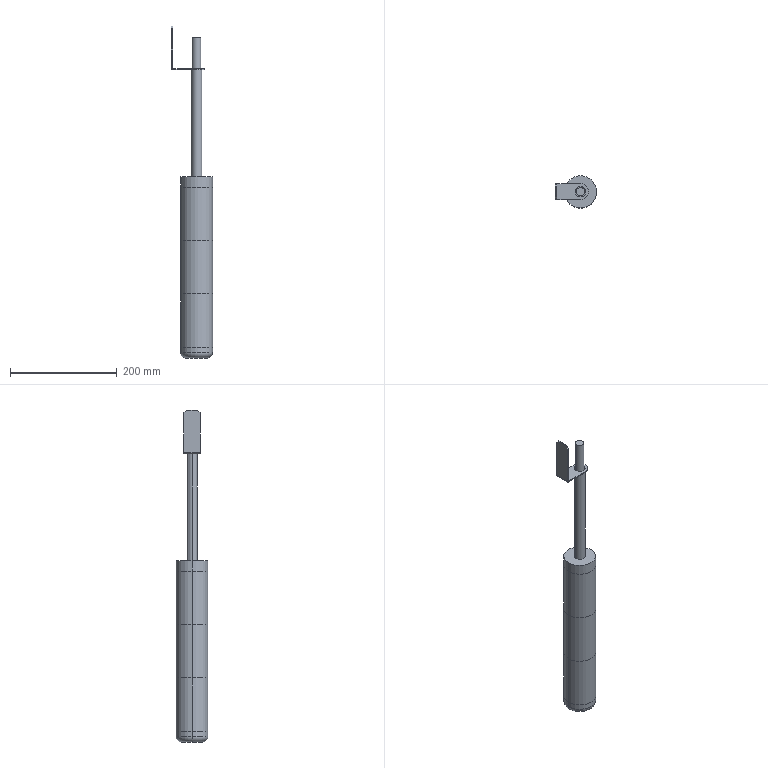Part | SolidWorks | features BaseBody 6 | 6 solids | 47 faces | box 77 x 60 x 622 mm | volume 1040083 mm3 | plane 25 | cylinder 20 | torus 2 | commonest cylinder face diameters 60 x10 20 x4 16 x2 30 x2 1.473 x1 5.473 x1
STEP:
#1=CARTESIAN_POINT('',(-20.,0.,0.));
#2=VERTEX_POINT('',#1);
#3=CARTESIAN_POINT('',(20.,0.,0.));
#4=VERTEX_POINT('',#3);
#5=CARTESIAN_POINT('',(0.,0.,0.));
#6=DIRECTION('',(0.,0.,-1.));
#7=DIRECTION('',(1.,0.,0.));
#8=AXIS2_PLACEMENT_3D('',#5,#6,#7);
#9=CIRCLE('',#8,20.);
#10=EDGE_CURVE('',#2,#4,#9,.T.);
#11=ORIENTED_EDGE('',*,*,#10,.F.);
#12=CARTESIAN_POINT('',(-30.,0.,10.));
#13=VERTEX_POINT('',#12);
#14=CARTESIAN_POINT('',(-20.,0.,10.));
#15=DIRECTION('',(0.,1.,0.));
#16=DIRECTION('',(-1.,0.,0.));
#17=AXIS2_PLACEMENT_3D('',#14,#15,#16);
#18=CIRCLE('',#17,10.);
#19=EDGE_CURVE('',#2,#13,#18,.T.);
#20=ORIENTED_EDGE('',*,*,#19,.T.);
#21=CARTESIAN_POINT('',(30.,0.,10.));
#22=VERTEX_POINT('',#21);
#23=CARTESIAN_POINT('',(0.,0.,10.));
#24=DIRECTION('',(0.,0.,1.));
#25=DIRECTION('',(1.,0.,0.));
#26=AXIS2_PLACEMENT_3D('',#23,#24,#25);
#27=CIRCLE('',#26,30.);
#28=EDGE_CURVE('',#22,#13,#27,.T.);
#29=ORIENTED_EDGE('',*,*,#28,.F.);
#30=CARTESIAN_POINT('',(20.,0.,10.));
#31=DIRECTION('',(0.,-1.,0.));
#32=DIRECTION('',(0.,0.,-1.));
#33=AXIS2_PLACEMENT_3D('',#30,#31,#32);
#34=CIRCLE('',#33,10.);
#35=EDGE_CURVE('',#4,#22,#34,.T.);
#36=ORIENTED_EDGE('',*,*,#35,.F.);
#37=EDGE_LOOP('',(#11,#20,#29,#36));
#38=FACE_OUTER_BOUND('',#37,.T.);
#39=CARTESIAN_POINT('',(0.,0.,10.));
#40=DIRECTION('',(0.,0.,1.));
#41=DIRECTION('',(1.,0.,0.));
#42=AXIS2_PLACEMENT_3D('',#39,#40,#41);
#43=TOROIDAL_SURFACE('',#42,20.,10.);
#44=ADVANCED_FACE('',(#38),#43,.T.);
#45=CARTESIAN_POINT('',(30.,0.,20.));
#46=VERTEX_POINT('',#45);
#47=CARTESIAN_POINT('',(-30.,0.,20.));
#48=VERTEX_POINT('',#47);
#49=CARTESIAN_POINT('',(0.,0.,20.));
#50=DIRECTION('',(0.,0.,1.));
#51=DIRECTION('',(1.,0.,0.));
#52=AXIS2_PLACEMENT_3D('',#49,#50,#51);
#53=CIRCLE('',#52,30.);
#54=EDGE_CURVE('',#46,#48,#53,.T.);
#55=ORIENTED_EDGE('',*,*,#54,.F.);
#56=CARTESIAN_POINT('',(30.,0.,20.));
#57=DIRECTION('',(0.,0.,-1.));
#58=VECTOR('',#57,1000.);
#59=LINE('',#56,#58);
#60=EDGE_CURVE('',#46,#22,#59,.T.);
#61=ORIENTED_EDGE('',*,*,#60,.T.);
#62=ORIENTED_EDGE('',*,*,#28,.T.);
#63=CARTESIAN_POINT('',(-30.,0.,20.));
#64=DIRECTION('',(0.,0.,-1.));
#65=VECTOR('',#64,1000.);
#66=LINE('',#63,#65);
#67=EDGE_CURVE('',#48,#13,#66,.T.);
#68=ORIENTED_EDGE('',*,*,#67,.F.);
#69=EDGE_LOOP('',(#55,#61,#62,#68));
#70=FACE_OUTER_BOUND('',#69,.T.);
#71=CARTESIAN_POINT('',(0.,0.,20.));
#72=DIRECTION('',(0.,0.,-1.));
#73=DIRECTION('',(-1.,0.,0.));
#74=AXIS2_PLACEMENT_3D('',#71,#72,#73);
#75=CYLINDRICAL_SURFACE('',#74,30.);
#76=ADVANCED_FACE('',(#70),#75,.T.);
#77=ORIENTED_EDGE('',*,*,#60,.F.);
#78=CARTESIAN_POINT('',(0.,0.,20.));
#79=DIRECTION('',(0.,0.,1.));
#80=DIRECTION('',(1.,0.,0.));
#81=AXIS2_PLACEMENT_3D('',#78,#79,#80);
#82=CIRCLE('',#81,30.);
#83=EDGE_CURVE('',#48,#46,#82,.T.);
#84=ORIENTED_EDGE('',*,*,#83,.F.);
#85=ORIENTED_EDGE('',*,*,#67,.T.);
#86=CARTESIAN_POINT('',(0.,0.,10.));
#87=DIRECTION('',(0.,0.,1.));
#88=DIRECTION('',(1.,0.,0.));
#89=AXIS2_PLACEMENT_3D('',#86,#87,#88);
#90=CIRCLE('',#89,30.);
#91=EDGE_CURVE('',#13,#22,#90,.T.);
#92=ORIENTED_EDGE('',*,*,#91,.T.);
#93=EDGE_LOOP('',(#77,#84,#85,#92));
#94=FACE_OUTER_BOUND('',#93,.T.);
#95=CARTESIAN_POINT('',(0.,0.,20.));
#96=DIRECTION('',(0.,0.,-1.));
#97=DIRECTION('',(-1.,0.,0.));
#98=AXIS2_PLACEMENT_3D('',#95,#96,#97);
#99=CYLINDRICAL_SURFACE('',#98,30.);
#100=ADVANCED_FACE('',(#94),#99,.T.);
#101=ORIENTED_EDGE('',*,*,#83,.T.);
#102=ORIENTED_EDGE('',*,*,#54,.T.);
#103=EDGE_LOOP('',(#101,#102));
#104=FACE_OUTER_BOUND('',#103,.T.);
#105=CARTESIAN_POINT('',(0.,0.,20.));
#106=DIRECTION('',(0.,0.,1.));
#107=DIRECTION('',(1.,0.,0.));
#108=AXIS2_PLACEMENT_3D('',#105,#106,#107);
#109=PLANE('',#108);
#110=ADVANCED_FACE('',(#104),#109,.T.);
#111=CARTESIAN_POINT('',(0.,0.,0.));
#112=DIRECTION('',(0.,0.,-1.));
#113=DIRECTION('',(1.,0.,0.));
#114=AXIS2_PLACEMENT_3D('',#111,#112,#113);
#115=CIRCLE('',#114,20.);
#116=EDGE_CURVE('',#4,#2,#115,.T.);
#117=ORIENTED_EDGE('',*,*,#116,.T.);
#118=ORIENTED_EDGE('',*,*,#10,.T.);
#119=EDGE_LOOP('',(#117,#118));
#120=FACE_OUTER_BOUND('',#119,.T.);
#121=CARTESIAN_POINT('',(0.,0.,0.));
#122=DIRECTION('',(0.,0.,1.));
#123=DIRECTION('',(1.,0.,0.));
#124=AXIS2_PLACEMENT_3D('',#121,#122,#123);
#125=PLANE('',#124);
#126=ADVANCED_FACE('',(#120),#125,.F.);
#127=ORIENTED_EDGE('',*,*,#19,.F.);
#128=ORIENTED_EDGE('',*,*,#116,.F.);
#129=ORIENTED_EDGE('',*,*,#35,.T.);
#130=ORIENTED_EDGE('',*,*,#91,.F.);
#131=EDGE_LOOP('',(#127,#128,#129,#130));
#132=FACE_OUTER_BOUND('',#131,.T.);
#133=CARTESIAN_POINT('',(0.,0.,10.));
#134=DIRECTION('',(0.,0.,1.));
#135=DIRECTION('',(1.,0.,0.));
#136=AXIS2_PLACEMENT_3D('',#133,#134,#135);
#137=TOROIDAL_SURFACE('',#136,20.,10.);
#138=ADVANCED_FACE('',(#132),#137,.T.);
#139=CLOSED_SHELL('',(#44,#76,#100,#110,#126,#138));
#140=MANIFOLD_SOLID_BREP('',#139);
#141=CARTESIAN_POINT('',(30.,0.,120.));
#142=VERTEX_POINT('',#141);
#143=CARTESIAN_POINT('',(-30.,0.,120.));
#144=VERTEX_POINT('',#143);
#145=CARTESIAN_POINT('',(0.,0.,120.));
#146=DIRECTION('',(0.,0.,1.));
#147=DIRECTION('',(1.,0.,0.));
#148=AXIS2_PLACEMENT_3D('',#145,#146,#147);
#149=CIRCLE('',#148,30.);
#150=EDGE_CURVE('',#142,#144,#149,.T.);
#151=ORIENTED_EDGE('',*,*,#150,.F.);
#152=CARTESIAN_POINT('',(30.,0.,20.));
#153=VERTEX_POINT('',#152);
#154=CARTESIAN_POINT('',(30.,0.,120.));
#155=DIRECTION('',(0.,0.,-1.));
#156=VECTOR('',#155,1000.);
#157=LINE('',#154,#156);
#158=EDGE_CURVE('',#142,#153,#157,.T.);
#159=ORIENTED_EDGE('',*,*,#158,.T.);
#160=CARTESIAN_POINT('',(-30.,0.,20.));
#161=VERTEX_POINT('',#160);
#162=CARTESIAN_POINT('',(0.,0.,20.));
#163=DIRECTION('',(0.,0.,1.));
#164=DIRECTION('',(1.,0.,0.));
#165=AXIS2_PLACEMENT_3D('',#162,#163,#164);
#166=CIRCLE('',#165,30.);
#167=EDGE_CURVE('',#153,#161,#166,.T.);
#168=ORIENTED_EDGE('',*,*,#167,.T.);
#169=CARTESIAN_POINT('',(-30.,0.,120.));
#170=DIRECTION('',(0.,0.,-1.));
#171=VECTOR('',#170,1000.);
#172=LINE('',#169,#171);
#173=EDGE_CURVE('',#144,#161,#172,.T.);
#174=ORIENTED_EDGE('',*,*,#173,.F.);
#175=EDGE_LOOP('',(#151,#159,#168,#174));
#176=FACE_OUTER_BOUND('',#175,.T.);
#177=CARTESIAN_POINT('',(0.,0.,120.));
#178=DIRECTION('',(0.,0.,-1.));
#179=DIRECTION('',(-1.,0.,0.));
#180=AXIS2_PLACEMENT_3D('',#177,#178,#179);
#181=CYLINDRICAL_SURFACE('',#180,30.);
#182=ADVANCED_FACE('',(#176),#181,.T.);
#183=ORIENTED_EDGE('',*,*,#158,.F.);
#184=CARTESIAN_POINT('',(0.,0.,120.));
#185=DIRECTION('',(0.,0.,1.));
#186=DIRECTION('',(1.,0.,0.));
#187=AXIS2_PLACEMENT_3D('',#184,#185,#186);
#188=CIRCLE('',#187,30.);
#189=EDGE_CURVE('',#144,#142,#188,.T.);
#190=ORIENTED_EDGE('',*,*,#189,.F.);
#191=ORIENTED_EDGE('',*,*,#173,.T.);
#192=CARTESIAN_POINT('',(0.,0.,20.));
#193=DIRECTION('',(0.,0.,1.));
#194=DIRECTION('',(1.,0.,0.));
#195=AXIS2_PLACEMENT_3D('',#192,#193,#194);
#196=CIRCLE('',#195,30.);
#197=EDGE_CURVE('',#161,#153,#196,.T.);
#198=ORIENTED_EDGE('',*,*,#197,.T.);
#199=EDGE_LOOP('',(#183,#190,#191,#198));
#200=FACE_OUTER_BOUND('',#199,.T.);
#201=CARTESIAN_POINT('',(0.,0.,120.));
#202=DIRECTION('',(0.,0.,-1.));
#203=DIRECTION('',(-1.,0.,0.));
#204=AXIS2_PLACEMENT_3D('',#201,#202,#203);
#205=CYLINDRICAL_SURFACE('',#204,30.);
#206=ADVANCED_FACE('',(#200),#205,.T.);
#207=ORIENTED_EDGE('',*,*,#189,.T.);
#208=ORIENTED_EDGE('',*,*,#150,.T.);
#209=EDGE_LOOP('',(#207,#208));
#210=FACE_OUTER_BOUND('',#209,.T.);
#211=CARTESIAN_POINT('',(0.,0.,120.));
#212=DIRECTION('',(0.,0.,1.));
#213=DIRECTION('',(1.,0.,0.));
#214=AXIS2_PLACEMENT_3D('',#211,#212,#213);
#215=PLANE('',#214);
#216=ADVANCED_FACE('',(#210),#215,.T.);
#217=ORIENTED_EDGE('',*,*,#197,.F.);
#218=ORIENTED_EDGE('',*,*,#167,.F.);
#219=EDGE_LOOP('',(#217,#218));
#220=FACE_OUTER_BOUND('',#219,.T.);
#221=CARTESIAN_POINT('',(0.,0.,20.));
#222=DIRECTION('',(0.,0.,1.));
#223=DIRECTION('',(1.,0.,0.));
#224=AXIS2_PLACEMENT_3D('',#221,#222,#223);
#225=PLANE('',#224);
#226=ADVANCED_FACE('',(#220),#225,.F.);
#227=CLOSED_SHELL('',(#182,#206,#216,#226));
#228=MANIFOLD_SOLID_BREP('',#227);
#229=CARTESIAN_POINT('',(30.,0.,220.));
#230=VERTEX_POINT('',#229);
#231=CARTESIAN_POINT('',(-30.,0.,220.));
#232=VERTEX_POINT('',#231);
#233=CARTESIAN_POINT('',(0.,0.,220.));
#234=DIRECTION('',(0.,0.,1.));
#235=DIRECTION('',(1.,0.,0.));
#236=AXIS2_PLACEMENT_3D('',#233,#234,#235);
#237=CIRCLE('',#236,30.);
#238=EDGE_CURVE('',#230,#232,#237,.T.);
#239=ORIENTED_EDGE('',*,*,#238,.F.);
#240=CARTESIAN_POINT('',(30.,0.,120.));
#241=VERTEX_POINT('',#240);
#242=CARTESIAN_POINT('',(30.,0.,220.));
#243=DIRECTION('',(0.,0.,-1.));
#244=VECTOR('',#243,1000.);
#245=LINE('',#242,#244);
#246=EDGE_CURVE('',#230,#241,#245,.T.);
#247=ORIENTED_EDGE('',*,*,#246,.T.);
#248=CARTESIAN_POINT('',(-30.,0.,120.));
#249=VERTEX_POINT('',#248);
#250=CARTESIAN_POINT('',(0.,0.,120.));
#251=DIRECTION('',(0.,0.,1.));
#252=DIRECTION('',(1.,0.,0.));
#253=AXIS2_PLACEMENT_3D('',#250,#251,#252);
#254=CIRCLE('',#253,30.);
#255=EDGE_CURVE('',#241,#249,#254,.T.);
#256=ORIENTED_EDGE('',*,*,#255,.T.);
#257=CARTESIAN_POINT('',(-30.,0.,220.));
#258=DIRECTION('',(0.,0.,-1.));
#259=VECTOR('',#258,1000.);
#260=LINE('',#257,#259);
#261=EDGE_CURVE('',#232,#249,#260,.T.);
#262=ORIENTED_EDGE('',*,*,#261,.F.);
#263=EDGE_LOOP('',(#239,#247,#256,#262));
#264=FACE_OUTER_BOUND('',#263,.T.);
#265=CARTESIAN_POINT('',(0.,0.,220.));
#266=DIRECTION('',(0.,0.,-1.));
#267=DIRECTION('',(-1.,0.,0.));
#268=AXIS2_PLACEMENT_3D('',#265,#266,#267);
#269=CYLINDRICAL_SURFACE('',#268,30.);
#270=ADVANCED_FACE('',(#264),#269,.T.);
#271=ORIENTED_EDGE('',*,*,#246,.F.);
#272=CARTESIAN_POINT('',(0.,0.,220.));
#273=DIRECTION('',(0.,0.,1.));
#274=DIRECTION('',(1.,0.,0.));
#275=AXIS2_PLACEMENT_3D('',#272,#273,#274);
#276=CIRCLE('',#275,30.);
#277=EDGE_CURVE('',#232,#230,#276,.T.);
#278=ORIENTED_EDGE('',*,*,#277,.F.);
#279=ORIENTED_EDGE('',*,*,#261,.T.);
#280=CARTESIAN_POINT('',(0.,0.,120.));
#281=DIRECTION('',(0.,0.,1.));
#282=DIRECTION('',(1.,0.,0.));
#283=AXIS2_PLACEMENT_3D('',#280,#281,#282);
#284=CIRCLE('',#283,30.);
#285=EDGE_CURVE('',#249,#241,#284,.T.);
#286=ORIENTED_EDGE('',*,*,#285,.T.);
#287=EDGE_LOOP('',(#271,#278,#279,#286));
#288=FACE_OUTER_BOUND('',#287,.T.);
#289=CARTESIAN_POINT('',(0.,0.,220.));
#290=DIRECTION('',(0.,0.,-1.));
#291=DIRECTION('',(-1.,0.,0.));
#292=AXIS2_PLACEMENT_3D('',#289,#290,#291);
#293=CYLINDRICAL_SURFACE('',#292,30.);
#294=ADVANCED_FACE('',(#288),#293,.T.);
#295=ORIENTED_EDGE('',*,*,#277,.T.);
#296=ORIENTED_EDGE('',*,*,#238,.T.);
#297=EDGE_LOOP('',(#295,#296));
#298=FACE_OUTER_BOUND('',#297,.T.);
#299=CARTESIAN_POINT('',(0.,0.,220.));
#300=DIRECTION('',(0.,0.,1.));
#301=DIRECTION('',(1.,0.,0.));
#302=AXIS2_PLACEMENT_3D('',#299,#300,#301);
#303=PLANE('',#302);
#304=ADVANCED_FACE('',(#298),#303,.T.);
#305=ORIENTED_EDGE('',*,*,#285,.F.);
#306=ORIENTED_EDGE('',*,*,#255,.F.);
#307=EDGE_LOOP('',(#305,#306));
#308=FACE_OUTER_BOUND('',#307,.T.);
#309=CARTESIAN_POINT('',(0.,0.,120.));
#310=DIRECTION('',(0.,0.,1.));
#311=DIRECTION('',(1.,0.,0.));
#312=AXIS2_PLACEMENT_3D('',#309,#310,#311);
#313=PLANE('',#312);
#314=ADVANCED_FACE('',(#308),#313,.F.);
#315=CLOSED_SHELL('',(#270,#294,#304,#314));
#316=MANIFOLD_SOLID_BREP('',#315);
#317=CARTESIAN_POINT('',(30.,0.,320.));
#318=VERTEX_POINT('',#317);
#319=CARTESIAN_POINT('',(-30.,0.,320.));
#320=VERTEX_POINT('',#319);
#321=CARTESIAN_POINT('',(0.,0.,320.));
#322=DIRECTION('',(0.,0.,1.));
#323=DIRECTION('',(1.,0.,0.));
#324=AXIS2_PLACEMENT_3D('',#321,#322,#323);
#325=CIRCLE('',#324,30.);
#326=EDGE_CURVE('',#318,#320,#325,.T.);
#327=ORIENTED_EDGE('',*,*,#326,.F.);
#328=CARTESIAN_POINT('',(30.,0.,220.));
#329=VERTEX_POINT('',#328);
#330=CARTESIAN_POINT('',(30.,0.,320.));
#331=DIRECTION('',(0.,0.,-1.));
#332=VECTOR('',#331,1000.);
#333=LINE('',#330,#332);
#334=EDGE_CURVE('',#318,#329,#333,.T.);
#335=ORIENTED_EDGE('',*,*,#334,.T.);
#336=CARTESIAN_POINT('',(-30.,0.,220.));
#337=VERTEX_POINT('',#336);
#338=CARTESIAN_POINT('',(0.,0.,220.));
#339=DIRECTION('',(0.,0.,1.));
#340=DIRECTION('',(1.,0.,0.));
#341=AXIS2_PLACEMENT_3D('',#338,#339,#340);
#342=CIRCLE('',#341,30.);
#343=EDGE_CURVE('',#329,#337,#342,.T.);
#344=ORIENTED_EDGE('',*,*,#343,.T.);
#345=CARTESIAN_POINT('',(-30.,0.,320.));
#346=DIRECTION('',(0.,0.,-1.));
#347=VECTOR('',#346,1000.);
#348=LINE('',#345,#347);
#349=EDGE_CURVE('',#320,#337,#348,.T.);
#350=ORIENTED_EDGE('',*,*,#349,.F.);
#351=EDGE_LOOP('',(#327,#335,#344,#350));
#352=FACE_OUTER_BOUND('',#351,.T.);
#353=CARTESIAN_POINT('',(0.,0.,320.));
#354=DIRECTION('',(0.,0.,-1.));
#355=DIRECTION('',(-1.,0.,0.));
#356=AXIS2_PLACEMENT_3D('',#353,#354,#355);
#357=CYLINDRICAL_SURFACE('',#356,30.);
#358=ADVANCED_FACE('',(#352),#357,.T.);
#359=ORIENTED_EDGE('',*,*,#334,.F.);
#360=CARTESIAN_POINT('',(0.,0.,320.));
#361=DIRECTION('',(0.,0.,1.));
#362=DIRECTION('',(1.,0.,0.));
#363=AXIS2_PLACEMENT_3D('',#360,#361,#362);
#364=CIRCLE('',#363,30.);
#365=EDGE_CURVE('',#320,#318,#364,.T.);
#366=ORIENTED_EDGE('',*,*,#365,.F.);
#367=ORIENTED_EDGE('',*,*,#349,.T.);
#368=CARTESIAN_POINT('',(0.,0.,220.));
#369=DIRECTION('',(0.,0.,1.));
#370=DIRECTION('',(1.,0.,0.));
#371=AXIS2_PLACEMENT_3D('',#368,#369,#370);
#372=CIRCLE('',#371,30.);
#373=EDGE_CURVE('',#337,#329,#372,.T.);
#374=ORIENTED_EDGE('',*,*,#373,.T.);
#375=EDGE_LOOP('',(#359,#366,#367,#374));
#376=FACE_OUTER_BOUND('',#375,.T.);
#377=CARTESIAN_POINT('',(0.,0.,320.));
#378=DIRECTION('',(0.,0.,-1.));
#379=DIRECTION('',(-1.,0.,0.));
#380=AXIS2_PLACEMENT_3D('',#377,#378,#379);
#381=CYLINDRICAL_SURFACE('',#380,30.);
#382=ADVANCED_FACE('',(#376),#381,.T.);
#383=ORIENTED_EDGE('',*,*,#365,.T.);
#384=ORIENTED_EDGE('',*,*,#326,.T.);
#385=EDGE_LOOP('',(#383,#384));
#386=FACE_OUTER_BOUND('',#385,.T.);
#387=CARTESIAN_POINT('',(0.,0.,320.));
#388=DIRECTION('',(0.,0.,1.));
#389=DIRECTION('',(1.,0.,0.));
#390=AXIS2_PLACEMENT_3D('',#387,#388,#389);
#391=PLANE('',#390);
#392=ADVANCED_FACE('',(#386),#391,.T.);
#393=ORIENTED_EDGE('',*,*,#373,.F.);
#394=ORIENTED_EDGE('',*,*,#343,.F.);
#395=EDGE_LOOP('',(#393,#394));
#396=FACE_OUTER_BOUND('',#395,.T.);
#397=CARTESIAN_POINT('',(0.,0.,220.));
#398=DIRECTION('',(0.,0.,1.));
#399=DIRECTION('',(1.,0.,0.));
#400=AXIS2_PLACEMENT_3D('',#397,#398,#399);
#401=PLANE('',#400);
#402=ADVANCED_FACE('',(#396),#401,.F.);
#403=CLOSED_SHELL('',(#358,#382,#392,#402));
#404=MANIFOLD_SOLID_BREP('',#403);
#405=CARTESIAN_POINT('',(8.,0.,600.));
#406=VERTEX_POINT('',#405);
#407=CARTESIAN_POINT('',(-8.,0.,600.));
#408=VERTEX_POINT('',#407);
#409=CARTESIAN_POINT('',(0.,0.,600.));
#410=DIRECTION('',(0.,0.,1.));
#411=DIRECTION('',(1.,0.,0.));
#412=AXIS2_PLACEMENT_3D('',#409,#410,#411);
#413=CIRCLE('',#412,8.);
#414=EDGE_CURVE('',#406,#408,#413,.T.);
#415=ORIENTED_EDGE('',*,*,#414,.F.);
#416=CARTESIAN_POINT('',(8.,0.,540.));
#417=VERTEX_POINT('',#416);
#418=CARTESIAN_POINT('',(8.,0.,600.));
#419=DIRECTION('',(0.,0.,-1.));
#420=VECTOR('',#419,1000.);
#421=LINE('',#418,#420);
#422=EDGE_CURVE('',#406,#417,#421,.T.);
#423=ORIENTED_EDGE('',*,*,#422,.T.);
#424=CARTESIAN_POINT('',(-8.,0.,540.));
#425=VERTEX_POINT('',#424);
#426=CARTESIAN_POINT('',(0.,0.,540.));
#427=DIRECTION('',(0.,0.,1.));
#428=DIRECTION('',(1.,0.,0.));
#429=AXIS2_PLACEMENT_3D('',#426,#427,#428);
#430=CIRCLE('',#429,8.);
#431=EDGE_CURVE('',#417,#425,#430,.T.);
#432=ORIENTED_EDGE('',*,*,#431,.T.);
#433=CARTESIAN_POINT('',(-8.,0.,600.));
#434=DIRECTION('',(0.,0.,-1.));
#435=VECTOR('',#434,1000.);
#436=LINE('',#433,#435);
#437=EDGE_CURVE('',#408,#425,#436,.T.);
#438=ORIENTED_EDGE('',*,*,#437,.F.);
#439=EDGE_LOOP('',(#415,#423,#432,#438));
#440=FACE_OUTER_BOUND('',#439,.T.);
#441=CARTESIAN_POINT('',(0.,0.,600.));
#442=DIRECTION('',(0.,0.,-1.));
#443=DIRECTION('',(-1.,0.,0.));
#444=AXIS2_PLACEMENT_3D('',#441,#442,#443);
#445=CYLINDRICAL_SURFACE('',#444,8.);
#446=ADVANCED_FACE('',(#440),#445,.T.);
#447=CARTESIAN_POINT('',(10.,0.,540.));
#448=VERTEX_POINT('',#447);
#449=CARTESIAN_POINT('',(-10.,0.,540.));
#450=VERTEX_POINT('',#449);
#451=CARTESIAN_POINT('',(0.,0.,540.));
#452=DIRECTION('',(0.,0.,1.));
#453=DIRECTION('',(1.,0.,0.));
#454=AXIS2_PLACEMENT_3D('',#451,#452,#453);
#455=CIRCLE('',#454,10.);
#456=EDGE_CURVE('',#448,#450,#455,.T.);
#457=ORIENTED_EDGE('',*,*,#456,.F.);
#458=CARTESIAN_POINT('',(10.,0.,340.));
#459=VERTEX_POINT('',#458);
#460=CARTESIAN_POINT('',(10.,0.,540.));
#461=DIRECTION('',(0.,0.,-1.));
#462=VECTOR('',#461,1000.);
#463=LINE('',#460,#462);
#464=EDGE_CURVE('',#448,#459,#463,.T.);
#465=ORIENTED_EDGE('',*,*,#464,.T.);
#466=CARTESIAN_POINT('',(-10.,0.,340.));
#467=VERTEX_POINT('',#466);
#468=CARTESIAN_POINT('',(0.,0.,340.));
#469=DIRECTION('',(0.,0.,1.));
#470=DIRECTION('',(1.,0.,0.));
#471=AXIS2_PLACEMENT_3D('',#468,#469,#470);
#472=CIRCLE('',#471,10.);
#473=EDGE_CURVE('',#459,#467,#472,.T.);
#474=ORIENTED_EDGE('',*,*,#473,.T.);
#475=CARTESIAN_POINT('',(-10.,0.,540.));
#476=DIRECTION('',(0.,0.,-1.));
#477=VECTOR('',#476,1000.);
#478=LINE('',#475,#477);
#479=EDGE_CURVE('',#450,#467,#478,.T.);
#480=ORIENTED_EDGE('',*,*,#479,.F.);
#481=EDGE_LOOP('',(#457,#465,#474,#480));
#482=FACE_OUTER_BOUND('',#481,.T.);
#483=CARTESIAN_POINT('',(0.,0.,540.));
#484=DIRECTION('',(0.,0.,-1.));
#485=DIRECTION('',(-1.,0.,0.));
#486=AXIS2_PLACEMENT_3D('',#483,#484,#485);
#487=CYLINDRICAL_SURFACE('',#486,10.);
#488=ADVANCED_FACE('',(#482),#487,.T.);
#489=CARTESIAN_POINT('',(30.,0.,340.));
#490=VERTEX_POINT('',#489);
#491=CARTESIAN_POINT('',(-30.,0.,340.));
#492=VERTEX_POINT('',#491);
#493=CARTESIAN_POINT('',(0.,0.,340.));
#494=DIRECTION('',(0.,0.,1.));
#495=DIRECTION('',(1.,0.,0.));
#496=AXIS2_PLACEMENT_3D('',#493,#494,#495);
#497=CIRCLE('',#496,30.);
#498=EDGE_CURVE('',#490,#492,#497,.T.);
#499=ORIENTED_EDGE('',*,*,#498,.F.);
#500=CARTESIAN_POINT('',(30.,0.,320.));
#501=VERTEX_POINT('',#500);
#502=CARTESIAN_POINT('',(30.,0.,340.));
#503=DIRECTION('',(0.,0.,-1.));
#504=VECTOR('',#503,1000.);
#505=LINE('',#502,#504);
#506=EDGE_CURVE('',#490,#501,#505,.T.);
#507=ORIENTED_EDGE('',*,*,#506,.T.);
#508=CARTESIAN_POINT('',(-30.,0.,320.));
#509=VERTEX_POINT('',#508);
#510=CARTESIAN_POINT('',(0.,0.,320.));
#511=DIRECTION('',(0.,0.,1.));
#512=DIRECTION('',(1.,0.,0.));
#513=AXIS2_PLACEMENT_3D('',#510,#511,#512);
#514=CIRCLE('',#513,30.);
#515=EDGE_CURVE('',#501,#509,#514,.T.);
#516=ORIENTED_EDGE('',*,*,#515,.T.);
#517=CARTESIAN_POINT('',(-30.,0.,340.));
#518=DIRECTION('',(0.,0.,-1.));
#519=VECTOR('',#518,1000.);
#520=LINE('',#517,#519);
#521=EDGE_CURVE('',#492,#509,#520,.T.);
#522=ORIENTED_EDGE('',*,*,#521,.F.);
#523=EDGE_LOOP('',(#499,#507,#516,#522));
#524=FACE_OUTER_BOUND('',#523,.T.);
#525=CARTESIAN_POINT('',(0.,0.,340.));
#526=DIRECTION('',(0.,0.,-1.));
#527=DIRECTION('',(-1.,0.,0.));
#528=AXIS2_PLACEMENT_3D('',#525,#526,#527);
#529=CYLINDRICAL_SURFACE('',#528,30.);
#530=ADVANCED_FACE('',(#524),#529,.T.);
#531=CARTESIAN_POINT('',(0.,0.,540.));
#532=DIRECTION('',(0.,0.,1.));
#533=DIRECTION('',(1.,0.,0.));
#534=AXIS2_PLACEMENT_3D('',#531,#532,#533);
#535=CIRCLE('',#534,10.);
#536=EDGE_CURVE('',#450,#448,#535,.T.);
#537=ORIENTED_EDGE('',*,*,#536,.T.);
#538=ORIENTED_EDGE('',*,*,#456,.T.);
#539=EDGE_LOOP('',(#537,#538));
#540=FACE_OUTER_BOUND('',#539,.T.);
#541=CARTESIAN_POINT('',(0.,0.,540.));
#542=DIRECTION('',(0.,0.,1.));
#543=DIRECTION('',(1.,0.,0.));
#544=AXIS2_PLACEMENT_3D('',#541,#542,#543);
#545=CIRCLE('',#544,8.);
#546=EDGE_CURVE('',#425,#417,#545,.T.);
#547=ORIENTED_EDGE('',*,*,#546,.F.);
#548=ORIENTED_EDGE('',*,*,#431,.F.);
#549=EDGE_LOOP('',(#547,#548));
#550=FACE_BOUND('',#549,.T.);
#551=CARTESIAN_POINT('',(0.,0.,540.));
#552=DIRECTION('',(0.,0.,1.));
#553=DIRECTION('',(1.,0.,0.));
#554=AXIS2_PLACEMENT_3D('',#551,#552,#553);
#555=PLANE('',#554);
#556=ADVANCED_FACE('',(#540,#550),#555,.T.);
#557=CARTESIAN_POINT('',(0.,0.,340.));
#558=DIRECTION('',(0.,0.,1.));
#559=DIRECTION('',(1.,0.,0.));
#560=AXIS2_PLACEMENT_3D('',#557,#558,#559);
#561=CIRCLE('',#560,30.);
#562=EDGE_CURVE('',#492,#490,#561,.T.);
#563=ORIENTED_EDGE('',*,*,#562,.T.);
#564=ORIENTED_EDGE('',*,*,#498,.T.);
#565=EDGE_LOOP('',(#563,#564));
#566=FACE_OUTER_BOUND('',#565,.T.);
#567=CARTESIAN_POINT('',(0.,0.,340.));
#568=DIRECTION('',(0.,0.,1.));
#569=DIRECTION('',(1.,0.,0.));
#570=AXIS2_PLACEMENT_3D('',#567,#568,#569);
#571=CIRCLE('',#570,10.);
#572=EDGE_CURVE('',#467,#459,#571,.T.);
#573=ORIENTED_EDGE('',*,*,#572,.F.);
#574=ORIENTED_EDGE('',*,*,#473,.F.);
#575=EDGE_LOOP('',(#573,#574));
#576=FACE_BOUND('',#575,.T.);
#577=CARTESIAN_POINT('',(0.,0.,340.));
#578=DIRECTION('',(0.,0.,1.));
#579=DIRECTION('',(1.,0.,0.));
#580=AXIS2_PLACEMENT_3D('',#577,#578,#579);
#581=PLANE('',#580);
#582=ADVANCED_FACE('',(#566,#576),#581,.T.);
#583=ORIENTED_EDGE('',*,*,#506,.F.);
#584=ORIENTED_EDGE('',*,*,#562,.F.);
#585=ORIENTED_EDGE('',*,*,#521,.T.);
#586=CARTESIAN_POINT('',(0.,0.,320.));
#587=DIRECTION('',(0.,0.,1.));
#588=DIRECTION('',(1.,0.,0.));
#589=AXIS2_PLACEMENT_3D('',#586,#587,#588);
#590=CIRCLE('',#589,30.);
#591=EDGE_CURVE('',#509,#501,#590,.T.);
#592=ORIENTED_EDGE('',*,*,#591,.T.);
#593=EDGE_LOOP('',(#583,#584,#585,#592));
#594=FACE_OUTER_BOUND('',#593,.T.);
#595=CARTESIAN_POINT('',(0.,0.,340.));
#596=DIRECTION('',(0.,0.,-1.));
#597=DIRECTION('',(-1.,0.,0.));
#598=AXIS2_PLACEMENT_3D('',#595,#596,#597);
#599=CYLINDRICAL_SURFACE('',#598,30.);
#600=ADVANCED_FACE('',(#594),#599,.T.);
#601=ORIENTED_EDGE('',*,*,#591,.F.);
#602=ORIENTED_EDGE('',*,*,#515,.F.);
#603=EDGE_LOOP('',(#601,#602));
#604=FACE_OUTER_BOUND('',#603,.T.);
#605=CARTESIAN_POINT('',(0.,0.,320.));
#606=DIRECTION('',(0.,0.,1.));
#607=DIRECTION('',(1.,0.,0.));
#608=AXIS2_PLACEMENT_3D('',#605,#606,#607);
#609=PLANE('',#608);
#610=ADVANCED_FACE('',(#604),#609,.F.);
#611=ORIENTED_EDGE('',*,*,#464,.F.);
#612=ORIENTED_EDGE('',*,*,#536,.F.);
#613=ORIENTED_EDGE('',*,*,#479,.T.);
#614=ORIENTED_EDGE('',*,*,#572,.T.);
#615=EDGE_LOOP('',(#611,#612,#613,#614));
#616=FACE_OUTER_BOUND('',#615,.T.);
#617=CARTESIAN_POINT('',(0.,0.,540.));
#618=DIRECTION('',(0.,0.,-1.));
#619=DIRECTION('',(-1.,0.,0.));
#620=AXIS2_PLACEMENT_3D('',#617,#618,#619);
#621=CYLINDRICAL_SURFACE('',#620,10.);
#622=ADVANCED_FACE('',(#616),#621,.T.);
#623=ORIENTED_EDGE('',*,*,#422,.F.);
#624=CARTESIAN_POINT('',(0.,0.,600.));
#625=DIRECTION('',(0.,0.,1.));
#626=DIRECTION('',(1.,0.,0.));
#627=AXIS2_PLACEMENT_3D('',#624,#625,#626);
#628=CIRCLE('',#627,8.);
#629=EDGE_CURVE('',#408,#406,#628,.T.);
#630=ORIENTED_EDGE('',*,*,#629,.F.);
#631=ORIENTED_EDGE('',*,*,#437,.T.);
#632=ORIENTED_EDGE('',*,*,#546,.T.);
#633=EDGE_LOOP('',(#623,#630,#631,#632));
#634=FACE_OUTER_BOUND('',#633,.T.);
#635=CARTESIAN_POINT('',(0.,0.,600.));
#636=DIRECTION('',(0.,0.,-1.));
#637=DIRECTION('',(-1.,0.,0.));
#638=AXIS2_PLACEMENT_3D('',#635,#636,#637);
#639=CYLINDRICAL_SURFACE('',#638,8.);
#640=ADVANCED_FACE('',(#634),#639,.T.);
#641=ORIENTED_EDGE('',*,*,#629,.T.);
#642=ORIENTED_EDGE('',*,*,#414,.T.);
#643=EDGE_LOOP('',(#641,#642));
#644=FACE_OUTER_BOUND('',#643,.T.);
#645=CARTESIAN_POINT('',(0.,0.,600.));
#646=DIRECTION('',(0.,0.,1.));
#647=DIRECTION('',(1.,0.,0.));
#648=AXIS2_PLACEMENT_3D('',#645,#646,#647);
#649=PLANE('',#648);
#650=ADVANCED_FACE('',(#644),#649,.T.);
#651=CLOSED_SHELL('',(#446,#488,#530,#556,#582,#600,#610,#622,#640,#650));
#652=MANIFOLD_SOLID_BREP('',#651);
#653=CARTESIAN_POINT('',(10.,0.,542.));
#654=VERTEX_POINT('',#653);
#655=CARTESIAN_POINT('',(-10.,0.,542.));
#656=VERTEX_POINT('',#655);
#657=CARTESIAN_POINT('',(0.,0.,542.));
#658=DIRECTION('',(0.,0.,1.));
#659=DIRECTION('',(-1.,0.,0.));
#660=AXIS2_PLACEMENT_3D('',#657,#658,#659);
#661=CIRCLE('',#660,10.);
#662=EDGE_CURVE('',#654,#656,#661,.T.);
#663=ORIENTED_EDGE('',*,*,#662,.T.);
#664=CARTESIAN_POINT('',(-10.,0.,540.));
#665=VERTEX_POINT('',#664);
#666=CARTESIAN_POINT('',(-10.,0.,622.));
#667=DIRECTION('',(0.,0.,-1.));
#668=VECTOR('',#667,1000.);
#669=LINE('',#666,#668);
#670=EDGE_CURVE('',#656,#665,#669,.T.);
#671=ORIENTED_EDGE('',*,*,#670,.T.);
#672=CARTESIAN_POINT('',(10.,0.,540.));
#673=VERTEX_POINT('',#672);
#674=CARTESIAN_POINT('',(0.,0.,540.));
#675=DIRECTION('',(0.,0.,-1.));
#676=DIRECTION('',(1.,0.,0.));
#677=AXIS2_PLACEMENT_3D('',#674,#675,#676);
#678=CIRCLE('',#677,10.);
#679=EDGE_CURVE('',#665,#673,#678,.T.);
#680=ORIENTED_EDGE('',*,*,#679,.T.);
#681=CARTESIAN_POINT('',(10.,0.,622.));
#682=DIRECTION('',(0.,0.,-1.));
#683=VECTOR('',#682,1000.);
#684=LINE('',#681,#683);
#685=EDGE_CURVE('',#654,#673,#684,.T.);
#686=ORIENTED_EDGE('',*,*,#685,.F.);
#687=EDGE_LOOP('',(#663,#671,#680,#686));
#688=FACE_OUTER_BOUND('',#687,.T.);
#689=CARTESIAN_POINT('',(0.,0.,622.));
#690=DIRECTION('',(0.,0.,-1.));
#691=DIRECTION('',(1.,0.,0.));
#692=AXIS2_PLACEMENT_3D('',#689,#690,#691);
#693=CYLINDRICAL_SURFACE('',#692,10.);
#694=ADVANCED_FACE('',(#688),#693,.F.);
#695=CARTESIAN_POINT('',(-45.,-15.,617.));
#696=VERTEX_POINT('',#695);
#697=CARTESIAN_POINT('',(-45.,-15.,542.737));
#698=VERTEX_POINT('',#697);
#699=CARTESIAN_POINT('',(-45.,-15.,542.));
#700=DIRECTION('',(0.,0.,-1.));
#701=VECTOR('',#700,1000.);
#702=LINE('',#699,#701);
#703=EDGE_CURVE('',#696,#698,#702,.T.);
#704=ORIENTED_EDGE('',*,*,#703,.F.);
#705=CARTESIAN_POINT('',(-47.,-15.,617.));
#706=VERTEX_POINT('',#705);
#707=CARTESIAN_POINT('',(-45.,-15.,617.));
#708=DIRECTION('',(-1.,0.,0.));
#709=VECTOR('',#708,1000.);
#710=LINE('',#707,#709);
#711=EDGE_CURVE('',#696,#706,#710,.T.);
#712=ORIENTED_EDGE('',*,*,#711,.T.);
#713=CARTESIAN_POINT('',(-47.,-15.,542.737));
#714=VERTEX_POINT('',#713);
#715=CARTESIAN_POINT('',(-47.,-15.,542.));
#716=DIRECTION('',(0.,0.,-1.));
#717=VECTOR('',#716,1000.);
#718=LINE('',#715,#717);
#719=EDGE_CURVE('',#706,#714,#718,.T.);
#720=ORIENTED_EDGE('',*,*,#719,.T.);
#721=CARTESIAN_POINT('',(-45.,-15.,542.737));
#722=DIRECTION('',(-1.,0.,0.));
#723=VECTOR('',#722,1000.);
#724=LINE('',#721,#723);
#725=EDGE_CURVE('',#698,#714,#724,.T.);
#726=ORIENTED_EDGE('',*,*,#725,.F.);
#727=EDGE_LOOP('',(#704,#712,#720,#726));
#728=FACE_OUTER_BOUND('',#727,.T.);
#729=CARTESIAN_POINT('',(-45.,-15.,542.));
#730=DIRECTION('',(0.,1.,0.));
#731=DIRECTION('',(-1.,0.,0.));
#732=AXIS2_PLACEMENT_3D('',#729,#730,#731);
#733=PLANE('',#732);
#734=ADVANCED_FACE('',(#728),#733,.F.);
#735=CARTESIAN_POINT('',(-47.,15.,542.737));
#736=VERTEX_POINT('',#735);
#737=CARTESIAN_POINT('',(-47.,15.,617.));
#738=VERTEX_POINT('',#737);
#739=CARTESIAN_POINT('',(-47.,15.,542.));
#740=DIRECTION('',(0.,0.,1.));
#741=VECTOR('',#740,1000.);
#742=LINE('',#739,#741);
#743=EDGE_CURVE('',#736,#738,#742,.T.);
#744=ORIENTED_EDGE('',*,*,#743,.T.);
#745=CARTESIAN_POINT('',(-45.,15.,617.));
#746=VERTEX_POINT('',#745);
#747=CARTESIAN_POINT('',(-45.,15.,617.));
#748=DIRECTION('',(1.,0.,0.));
#749=VECTOR('',#748,1000.);
#750=LINE('',#747,#749);
#751=EDGE_CURVE('',#738,#746,#750,.T.);
#752=ORIENTED_EDGE('',*,*,#751,.T.);
#753=CARTESIAN_POINT('',(-45.,15.,542.737));
#754=VERTEX_POINT('',#753);
#755=CARTESIAN_POINT('',(-45.,15.,542.));
#756=DIRECTION('',(0.,0.,1.));
#757=VECTOR('',#756,1000.);
#758=LINE('',#755,#757);
#759=EDGE_CURVE('',#754,#746,#758,.T.);
#760=ORIENTED_EDGE('',*,*,#759,.F.);
#761=CARTESIAN_POINT('',(-45.,15.,542.737));
#762=DIRECTION('',(-1.,0.,0.));
#763=VECTOR('',#762,1000.);
#764=LINE('',#761,#763);
#765=EDGE_CURVE('',#754,#736,#764,.T.);
#766=ORIENTED_EDGE('',*,*,#765,.T.);
#767=EDGE_LOOP('',(#744,#752,#760,#766));
#768=FACE_OUTER_BOUND('',#767,.T.);
#769=CARTESIAN_POINT('',(-45.,15.,542.));
#770=DIRECTION('',(0.,-1.,0.));
#771=DIRECTION('',(1.,0.,0.));
#772=AXIS2_PLACEMENT_3D('',#769,#770,#771);
#773=PLANE('',#772);
#774=ADVANCED_FACE('',(#768),#773,.F.);
#775=CARTESIAN_POINT('',(-45.,10.,622.));
#776=VERTEX_POINT('',#775);
#777=CARTESIAN_POINT('',(-45.,-10.,622.));
#778=VERTEX_POINT('',#777);
#779=CARTESIAN_POINT('',(-45.,-15.,622.));
#780=DIRECTION('',(0.,-1.,0.));
#781=VECTOR('',#780,1000.);
#782=LINE('',#779,#781);
#783=EDGE_CURVE('',#776,#778,#782,.T.);
#784=ORIENTED_EDGE('',*,*,#783,.T.);
#785=CARTESIAN_POINT('',(-45.,2.5,634.5));
#786=DIRECTION('',(0.,-0.7071,-0.7071));
#787=VECTOR('',#786,1000.);
#788=LINE('',#785,#787);
#789=EDGE_CURVE('',#778,#696,#788,.T.);
#790=ORIENTED_EDGE('',*,*,#789,.T.);
#791=ORIENTED_EDGE('',*,*,#703,.T.);
#792=CARTESIAN_POINT('',(-45.,15.,542.737));
#793=DIRECTION('',(0.,-1.,0.));
#794=VECTOR('',#793,1000.);
#795=LINE('',#792,#794);
#796=EDGE_CURVE('',#754,#698,#795,.T.);
#797=ORIENTED_EDGE('',*,*,#796,.F.);
#798=ORIENTED_EDGE('',*,*,#759,.T.);
#799=CARTESIAN_POINT('',(-45.,12.5,619.5));
#800=DIRECTION('',(0.,-0.7071,0.7071));
#801=VECTOR('',#800,1000.);
#802=LINE('',#799,#801);
#803=EDGE_CURVE('',#746,#776,#802,.T.);
#804=ORIENTED_EDGE('',*,*,#803,.T.);
#805=EDGE_LOOP('',(#784,#790,#791,#797,#798,#804));
#806=FACE_OUTER_BOUND('',#805,.T.);
#807=CARTESIAN_POINT('',(-45.,15.,622.));
#808=DIRECTION('',(1.,0.,0.));
#809=DIRECTION('',(0.,0.,1.));
#810=AXIS2_PLACEMENT_3D('',#807,#808,#809);
#811=PLANE('',#810);
#812=ADVANCED_FACE('',(#806),#811,.T.);
#813=ORIENTED_EDGE('',*,*,#719,.F.);
#814=CARTESIAN_POINT('',(-47.,-10.,622.));
#815=VERTEX_POINT('',#814);
#816=CARTESIAN_POINT('',(-47.,-15.,617.));
#817=DIRECTION('',(0.,0.7071,0.7071));
#818=VECTOR('',#817,1000.);
#819=LINE('',#816,#818);
#820=EDGE_CURVE('',#706,#815,#819,.T.);
#821=ORIENTED_EDGE('',*,*,#820,.T.);
#822=CARTESIAN_POINT('',(-47.,10.,622.));
#823=VERTEX_POINT('',#822);
#824=CARTESIAN_POINT('',(-47.,-15.,622.));
#825=DIRECTION('',(0.,-1.,0.));
#826=VECTOR('',#825,1000.);
#827=LINE('',#824,#826);
#828=EDGE_CURVE('',#823,#815,#827,.T.);
#829=ORIENTED_EDGE('',*,*,#828,.F.);
#830=CARTESIAN_POINT('',(-47.,10.,622.));
#831=DIRECTION('',(0.,0.7071,-0.7071));
#832=VECTOR('',#831,1000.);
#833=LINE('',#830,#832);
#834=EDGE_CURVE('',#823,#738,#833,.T.);
#835=ORIENTED_EDGE('',*,*,#834,.T.);
#836=ORIENTED_EDGE('',*,*,#743,.F.);
#837=CARTESIAN_POINT('',(-47.,15.,542.737));
#838=DIRECTION('',(0.,-1.,0.));
#839=VECTOR('',#838,1000.);
#840=LINE('',#837,#839);
#841=EDGE_CURVE('',#736,#714,#840,.T.);
#842=ORIENTED_EDGE('',*,*,#841,.T.);
#843=EDGE_LOOP('',(#813,#821,#829,#835,#836,#842));
#844=FACE_OUTER_BOUND('',#843,.T.);
#845=CARTESIAN_POINT('',(-47.,15.,622.));
#846=DIRECTION('',(1.,0.,0.));
#847=DIRECTION('',(0.,0.,1.));
#848=AXIS2_PLACEMENT_3D('',#845,#846,#847);
#849=PLANE('',#848);
#850=ADVANCED_FACE('',(#844),#849,.F.);
#851=ORIENTED_EDGE('',*,*,#828,.T.);
#852=CARTESIAN_POINT('',(-45.,-10.,622.));
#853=DIRECTION('',(1.,0.,0.));
#854=VECTOR('',#853,1000.);
#855=LINE('',#852,#854);
#856=EDGE_CURVE('',#815,#778,#855,.T.);
#857=ORIENTED_EDGE('',*,*,#856,.T.);
#858=ORIENTED_EDGE('',*,*,#783,.F.);
#859=CARTESIAN_POINT('',(-45.,10.,622.));
#860=DIRECTION('',(-1.,0.,0.));
#861=VECTOR('',#860,1000.);
#862=LINE('',#859,#861);
#863=EDGE_CURVE('',#776,#823,#862,.T.);
#864=ORIENTED_EDGE('',*,*,#863,.T.);
#865=EDGE_LOOP('',(#851,#857,#858,#864));
#866=FACE_OUTER_BOUND('',#865,.T.);
#867=CARTESIAN_POINT('',(-45.,-15.,622.));
#868=DIRECTION('',(0.,0.,-1.));
#869=DIRECTION('',(0.,1.,0.));
#870=AXIS2_PLACEMENT_3D('',#867,#868,#869);
#871=PLANE('',#870);
#872=ADVANCED_FACE('',(#866),#871,.F.);
#873=CARTESIAN_POINT('',(-44.263,-15.,542.));
#874=VERTEX_POINT('',#873);
#875=CARTESIAN_POINT('',(-44.263,-15.,540.));
#876=VERTEX_POINT('',#875);
#877=CARTESIAN_POINT('',(-44.263,-15.,542.));
#878=DIRECTION('',(0.,0.,-1.));
#879=VECTOR('',#878,1000.);
#880=LINE('',#877,#879);
#881=EDGE_CURVE('',#874,#876,#880,.T.);
#882=ORIENTED_EDGE('',*,*,#881,.F.);
#883=CARTESIAN_POINT('',(-44.263,-15.,542.737));
#884=DIRECTION('',(0.,-1.,0.));
#885=DIRECTION('',(-1.,0.,0.));
#886=AXIS2_PLACEMENT_3D('',#883,#884,#885);
#887=CIRCLE('',#886,0.7366);
#888=EDGE_CURVE('',#698,#874,#887,.T.);
#889=ORIENTED_EDGE('',*,*,#888,.F.);
#890=ORIENTED_EDGE('',*,*,#725,.T.);
#891=CARTESIAN_POINT('',(-44.263,-15.,542.737));
#892=DIRECTION('',(0.,-1.,0.));
#893=DIRECTION('',(-1.,0.,0.));
#894=AXIS2_PLACEMENT_3D('',#891,#892,#893);
#895=CIRCLE('',#894,2.737);
#896=EDGE_CURVE('',#714,#876,#895,.T.);
#897=ORIENTED_EDGE('',*,*,#896,.T.);
#898=EDGE_LOOP('',(#882,#889,#890,#897));
#899=FACE_OUTER_BOUND('',#898,.T.);
#900=CARTESIAN_POINT('',(-44.263,-15.,542.737));
#901=DIRECTION('',(0.,-1.,0.));
#902=DIRECTION('',(1.,0.,0.));
#903=AXIS2_PLACEMENT_3D('',#900,#901,#902);
#904=PLANE('',#903);
#905=ADVANCED_FACE('',(#899),#904,.T.);
#906=ORIENTED_EDGE('',*,*,#841,.F.);
#907=CARTESIAN_POINT('',(-44.263,15.,540.));
#908=VERTEX_POINT('',#907);
#909=CARTESIAN_POINT('',(-44.263,15.,542.737));
#910=DIRECTION('',(0.,1.,0.));
#911=DIRECTION('',(-1.,0.,0.));
#912=AXIS2_PLACEMENT_3D('',#909,#910,#911);
#913=CIRCLE('',#912,2.737);
#914=EDGE_CURVE('',#908,#736,#913,.T.);
#915=ORIENTED_EDGE('',*,*,#914,.F.);
#916=CARTESIAN_POINT('',(-44.263,-15.,540.));
#917=DIRECTION('',(0.,-1.,0.));
#918=VECTOR('',#917,1000.);
#919=LINE('',#916,#918);
#920=EDGE_CURVE('',#908,#876,#919,.T.);
#921=ORIENTED_EDGE('',*,*,#920,.T.);
#922=ORIENTED_EDGE('',*,*,#896,.F.);
#923=EDGE_LOOP('',(#906,#915,#921,#922));
#924=FACE_OUTER_BOUND('',#923,.T.);
#925=CARTESIAN_POINT('',(-44.263,15.,542.737));
#926=DIRECTION('',(0.,1.,0.));
#927=DIRECTION('',(0.,0.,-1.));
#928=AXIS2_PLACEMENT_3D('',#925,#926,#927);
#929=CYLINDRICAL_SURFACE('',#928,2.737);
#930=ADVANCED_FACE('',(#924),#929,.T.);
#931=CARTESIAN_POINT('',(-44.263,15.,542.));
#932=VERTEX_POINT('',#931);
#933=CARTESIAN_POINT('',(-44.263,15.,542.737));
#934=DIRECTION('',(0.,1.,0.));
#935=DIRECTION('',(-1.,0.,0.));
#936=AXIS2_PLACEMENT_3D('',#933,#934,#935);
#937=CIRCLE('',#936,0.7366);
#938=EDGE_CURVE('',#932,#754,#937,.T.);
#939=ORIENTED_EDGE('',*,*,#938,.F.);
#940=CARTESIAN_POINT('',(-44.263,15.,542.));
#941=DIRECTION('',(0.,0.,-1.));
#942=VECTOR('',#941,1000.);
#943=LINE('',#940,#942);
#944=EDGE_CURVE('',#932,#908,#943,.T.);
#945=ORIENTED_EDGE('',*,*,#944,.T.);
#946=ORIENTED_EDGE('',*,*,#914,.T.);
#947=ORIENTED_EDGE('',*,*,#765,.F.);
#948=EDGE_LOOP('',(#939,#945,#946,#947));
#949=FACE_OUTER_BOUND('',#948,.T.);
#950=CARTESIAN_POINT('',(-44.263,15.,542.737));
#951=DIRECTION('',(0.,-1.,0.));
#952=DIRECTION('',(1.,0.,0.));
#953=AXIS2_PLACEMENT_3D('',#950,#951,#952);
#954=PLANE('',#953);
#955=ADVANCED_FACE('',(#949),#954,.F.);
#956=ORIENTED_EDGE('',*,*,#796,.T.);
#957=ORIENTED_EDGE('',*,*,#888,.T.);
#958=CARTESIAN_POINT('',(-44.263,-15.,542.));
#959=DIRECTION('',(0.,1.,0.));
#960=VECTOR('',#959,1000.);
#961=LINE('',#958,#960);
#962=EDGE_CURVE('',#874,#932,#961,.T.);
#963=ORIENTED_EDGE('',*,*,#962,.T.);
#964=ORIENTED_EDGE('',*,*,#938,.T.);
#965=EDGE_LOOP('',(#956,#957,#963,#964));
#966=FACE_OUTER_BOUND('',#965,.T.);
#967=CARTESIAN_POINT('',(-44.263,15.,542.737));
#968=DIRECTION('',(0.,1.,0.));
#969=DIRECTION('',(0.,0.,-1.));
#970=AXIS2_PLACEMENT_3D('',#967,#968,#969);
#971=CYLINDRICAL_SURFACE('',#970,0.7366);
#972=ADVANCED_FACE('',(#966),#971,.F.);
#973=CARTESIAN_POINT('',(0.,-15.,540.));
#974=VERTEX_POINT('',#973);
#975=CARTESIAN_POINT('',(-45.,-15.,540.));
#976=DIRECTION('',(-1.,0.,0.));
#977=VECTOR('',#976,1000.);
#978=LINE('',#975,#977);
#979=EDGE_CURVE('',#974,#876,#978,.T.);
#980=ORIENTED_EDGE('',*,*,#979,.F.);
#981=CARTESIAN_POINT('',(0.,-15.,542.));
#982=VERTEX_POINT('',#981);
#983=CARTESIAN_POINT('',(0.,-15.,540.));
#984=DIRECTION('',(0.,0.,1.));
#985=VECTOR('',#984,1000.);
#986=LINE('',#983,#985);
#987=EDGE_CURVE('',#974,#982,#986,.T.);
#988=ORIENTED_EDGE('',*,*,#987,.T.);
#989=CARTESIAN_POINT('',(-45.,-15.,542.));
#990=DIRECTION('',(-1.,0.,0.));
#991=VECTOR('',#990,1000.);
#992=LINE('',#989,#991);
#993=EDGE_CURVE('',#982,#874,#992,.T.);
#994=ORIENTED_EDGE('',*,*,#993,.T.);
#995=ORIENTED_EDGE('',*,*,#881,.T.);
#996=EDGE_LOOP('',(#980,#988,#994,#995));
#997=FACE_OUTER_BOUND('',#996,.T.);
#998=CARTESIAN_POINT('',(-45.,-15.,540.));
#999=DIRECTION('',(0.,1.,0.));
#1000=DIRECTION('',(0.,0.,1.));
#1001=AXIS2_PLACEMENT_3D('',#998,#999,#1000);
#1002=PLANE('',#1001);
#1003=ADVANCED_FACE('',(#997),#1002,.F.);
#1004=CARTESIAN_POINT('',(0.,15.,542.));
#1005=VERTEX_POINT('',#1004);
#1006=CARTESIAN_POINT('',(15.,15.,542.));
#1007=DIRECTION('',(1.,0.,0.));
#1008=VECTOR('',#1007,1000.);
#1009=LINE('',#1006,#1008);
#1010=EDGE_CURVE('',#932,#1005,#1009,.T.);
#1011=ORIENTED_EDGE('',*,*,#1010,.T.);
#1012=CARTESIAN_POINT('',(0.,15.,540.));
#1013=VERTEX_POINT('',#1012);
#1014=CARTESIAN_POINT('',(0.,15.,540.));
#1015=DIRECTION('',(0.,0.,-1.));
#1016=VECTOR('',#1015,1000.);
#1017=LINE('',#1014,#1016);
#1018=EDGE_CURVE('',#1005,#1013,#1017,.T.);
#1019=ORIENTED_EDGE('',*,*,#1018,.T.);
#1020=CARTESIAN_POINT('',(15.,15.,540.));
#1021=DIRECTION('',(1.,0.,0.));
#1022=VECTOR('',#1021,1000.);
#1023=LINE('',#1020,#1022);
#1024=EDGE_CURVE('',#908,#1013,#1023,.T.);
#1025=ORIENTED_EDGE('',*,*,#1024,.F.);
#1026=ORIENTED_EDGE('',*,*,#944,.F.);
#1027=EDGE_LOOP('',(#1011,#1019,#1025,#1026));
#1028=FACE_OUTER_BOUND('',#1027,.T.);
#1029=CARTESIAN_POINT('',(15.,15.,540.));
#1030=DIRECTION('',(0.,-1.,0.));
#1031=DIRECTION('',(0.,0.,-1.));
#1032=AXIS2_PLACEMENT_3D('',#1029,#1030,#1031);
#1033=PLANE('',#1032);
#1034=ADVANCED_FACE('',(#1028),#1033,.F.);
#1035=CARTESIAN_POINT('',(0.,0.,540.));
#1036=DIRECTION('',(0.,0.,-1.));
#1037=DIRECTION('',(1.,0.,0.));
#1038=AXIS2_PLACEMENT_3D('',#1035,#1036,#1037);
#1039=CIRCLE('',#1038,10.);
#1040=EDGE_CURVE('',#673,#665,#1039,.T.);
#1041=ORIENTED_EDGE('',*,*,#1040,.F.);
#1042=ORIENTED_EDGE('',*,*,#679,.F.);
#1043=EDGE_LOOP('',(#1041,#1042));
#1044=FACE_BOUND('',#1043,.T.);
#1045=CARTESIAN_POINT('',(15.,0.,540.));
#1046=VERTEX_POINT('',#1045);
#1047=CARTESIAN_POINT('',(0.,0.,540.));
#1048=DIRECTION('',(0.,0.,-1.));
#1049=DIRECTION('',(-1.,0.,0.));
#1050=AXIS2_PLACEMENT_3D('',#1047,#1048,#1049);
#1051=CIRCLE('',#1050,15.);
#1052=EDGE_CURVE('',#1013,#1046,#1051,.T.);
#1053=ORIENTED_EDGE('',*,*,#1052,.T.);
#1054=CARTESIAN_POINT('',(0.,0.,540.));
#1055=DIRECTION('',(0.,0.,-1.));
#1056=DIRECTION('',(-1.,0.,0.));
#1057=AXIS2_PLACEMENT_3D('',#1054,#1055,#1056);
#1058=CIRCLE('',#1057,15.);
#1059=EDGE_CURVE('',#1046,#974,#1058,.T.);
#1060=ORIENTED_EDGE('',*,*,#1059,.T.);
#1061=ORIENTED_EDGE('',*,*,#979,.T.);
#1062=ORIENTED_EDGE('',*,*,#920,.F.);
#1063=ORIENTED_EDGE('',*,*,#1024,.T.);
#1064=EDGE_LOOP('',(#1053,#1060,#1061,#1062,#1063));
#1065=FACE_OUTER_BOUND('',#1064,.T.);
#1066=CARTESIAN_POINT('',(15.,-15.,540.));
#1067=DIRECTION('',(0.,0.,1.));
#1068=DIRECTION('',(-1.,0.,0.));
#1069=AXIS2_PLACEMENT_3D('',#1066,#1067,#1068);
#1070=PLANE('',#1069);
#1071=ADVANCED_FACE('',(#1044,#1065),#1070,.F.);
#1072=ORIENTED_EDGE('',*,*,#662,.F.);
#1073=CARTESIAN_POINT('',(0.,0.,542.));
#1074=DIRECTION('',(0.,0.,1.));
#1075=DIRECTION('',(-1.,0.,0.));
#1076=AXIS2_PLACEMENT_3D('',#1073,#1074,#1075);
#1077=CIRCLE('',#1076,10.);
#1078=EDGE_CURVE('',#656,#654,#1077,.T.);
#1079=ORIENTED_EDGE('',*,*,#1078,.F.);
#1080=EDGE_LOOP('',(#1072,#1079));
#1081=FACE_BOUND('',#1080,.T.);
#1082=ORIENTED_EDGE('',*,*,#993,.F.);
#1083=CARTESIAN_POINT('',(15.,0.,542.));
#1084=VERTEX_POINT('',#1083);
#1085=CARTESIAN_POINT('',(0.,0.,542.));
#1086=DIRECTION('',(0.,0.,1.));
#1087=DIRECTION('',(-1.,0.,0.));
#1088=AXIS2_PLACEMENT_3D('',#1085,#1086,#1087);
#1089=CIRCLE('',#1088,15.);
#1090=EDGE_CURVE('',#982,#1084,#1089,.T.);
#1091=ORIENTED_EDGE('',*,*,#1090,.T.);
#1092=CARTESIAN_POINT('',(0.,0.,542.));
#1093=DIRECTION('',(0.,0.,1.));
#1094=DIRECTION('',(-1.,0.,0.));
#1095=AXIS2_PLACEMENT_3D('',#1092,#1093,#1094);
#1096=CIRCLE('',#1095,15.);
#1097=EDGE_CURVE('',#1084,#1005,#1096,.T.);
#1098=ORIENTED_EDGE('',*,*,#1097,.T.);
#1099=ORIENTED_EDGE('',*,*,#1010,.F.);
#1100=ORIENTED_EDGE('',*,*,#962,.F.);
#1101=EDGE_LOOP('',(#1082,#1091,#1098,#1099,#1100));
#1102=FACE_OUTER_BOUND('',#1101,.T.);
#1103=CARTESIAN_POINT('',(15.,-15.,542.));
#1104=DIRECTION('',(0.,0.,1.));
#1105=DIRECTION('',(-1.,0.,0.));
#1106=AXIS2_PLACEMENT_3D('',#1103,#1104,#1105);
#1107=PLANE('',#1106);
#1108=ADVANCED_FACE('',(#1081,#1102),#1107,.T.);
#1109=CARTESIAN_POINT('',(15.,0.,540.));
#1110=DIRECTION('',(0.,0.,1.));
#1111=VECTOR('',#1110,1000.);
#1112=LINE('',#1109,#1111);
#1113=EDGE_CURVE('',#1046,#1084,#1112,.T.);
#1114=ORIENTED_EDGE('',*,*,#1113,.F.);
#1115=ORIENTED_EDGE('',*,*,#1052,.F.);
#1116=ORIENTED_EDGE('',*,*,#1018,.F.);
#1117=ORIENTED_EDGE('',*,*,#1097,.F.);
#1118=EDGE_LOOP('',(#1114,#1115,#1116,#1117));
#1119=FACE_OUTER_BOUND('',#1118,.T.);
#1120=CARTESIAN_POINT('',(0.,0.,540.));
#1121=DIRECTION('',(0.,0.,1.));
#1122=DIRECTION('',(-1.,0.,0.));
#1123=AXIS2_PLACEMENT_3D('',#1120,#1121,#1122);
#1124=CYLINDRICAL_SURFACE('',#1123,15.);
#1125=ADVANCED_FACE('',(#1119),#1124,.T.);
#1126=ORIENTED_EDGE('',*,*,#1059,.F.);
#1127=ORIENTED_EDGE('',*,*,#1113,.T.);
#1128=ORIENTED_EDGE('',*,*,#1090,.F.);
#1129=ORIENTED_EDGE('',*,*,#987,.F.);
#1130=EDGE_LOOP('',(#1126,#1127,#1128,#1129));
#1131=FACE_OUTER_BOUND('',#1130,.T.);
#1132=CARTESIAN_POINT('',(0.,0.,540.));
#1133=DIRECTION('',(0.,0.,1.));
#1134=DIRECTION('',(-1.,0.,0.));
#1135=AXIS2_PLACEMENT_3D('',#1132,#1133,#1134);
#1136=CYLINDRICAL_SURFACE('',#1135,15.);
#1137=ADVANCED_FACE('',(#1131),#1136,.T.);
#1138=ORIENTED_EDGE('',*,*,#789,.F.);
#1139=ORIENTED_EDGE('',*,*,#856,.F.);
#1140=ORIENTED_EDGE('',*,*,#820,.F.);
#1141=ORIENTED_EDGE('',*,*,#711,.F.);
#1142=EDGE_LOOP('',(#1138,#1139,#1140,#1141));
#1143=FACE_OUTER_BOUND('',#1142,.T.);
#1144=CARTESIAN_POINT('',(-45.,-15.,617.));
#1145=DIRECTION('',(0.,0.7071,-0.7071));
#1146=DIRECTION('',(0.,0.7071,0.7071));
#1147=AXIS2_PLACEMENT_3D('',#1144,#1145,#1146);
#1148=PLANE('',#1147);
#1149=ADVANCED_FACE('',(#1143),#1148,.F.);
#1150=ORIENTED_EDGE('',*,*,#803,.F.);
#1151=ORIENTED_EDGE('',*,*,#751,.F.);
#1152=ORIENTED_EDGE('',*,*,#834,.F.);
#1153=ORIENTED_EDGE('',*,*,#863,.F.);
#1154=EDGE_LOOP('',(#1150,#1151,#1152,#1153));
#1155=FACE_OUTER_BOUND('',#1154,.T.);
#1156=CARTESIAN_POINT('',(-45.,10.,622.));
#1157=DIRECTION('',(0.,-0.7071,-0.7071));
#1158=DIRECTION('',(0.,0.7071,-0.7071));
#1159=AXIS2_PLACEMENT_3D('',#1156,#1157,#1158);
#1160=PLANE('',#1159);
#1161=ADVANCED_FACE('',(#1155),#1160,.F.);
#1162=ORIENTED_EDGE('',*,*,#670,.F.);
#1163=ORIENTED_EDGE('',*,*,#1078,.T.);
#1164=ORIENTED_EDGE('',*,*,#685,.T.);
#1165=ORIENTED_EDGE('',*,*,#1040,.T.);
#1166=EDGE_LOOP('',(#1162,#1163,#1164,#1165));
#1167=FACE_OUTER_BOUND('',#1166,.T.);
#1168=CARTESIAN_POINT('',(0.,0.,622.));
#1169=DIRECTION('',(0.,0.,-1.));
#1170=DIRECTION('',(1.,0.,0.));
#1171=AXIS2_PLACEMENT_3D('',#1168,#1169,#1170);
#1172=CYLINDRICAL_SURFACE('',#1171,10.);
#1173=ADVANCED_FACE('',(#1167),#1172,.F.);
#1174=CLOSED_SHELL('',(#694,#734,#774,#812,#850,#872,#905,#930,#955,#972,#1003,#1034,#1071,#1108,#1125,#1137,#1149,#1161,#1173));
#1175=MANIFOLD_SOLID_BREP('',#1174);
#1176=CARTESIAN_POINT('',(0.,0.,0.));
#1177=DIRECTION('',(0.,0.,1.));
#1178=DIRECTION('',(1.,0.,0.));
#1179=AXIS2_PLACEMENT_3D('',#1176,#1177,#1178);
#1180=(LENGTH_UNIT()NAMED_UNIT(*)SI_UNIT(.MILLI.,.METRE.));
#1181=UNCERTAINTY_MEASURE_WITH_UNIT(LENGTH_MEASURE(0.00001),#1180,'','');
#1182=(NAMED_UNIT(*)PLANE_ANGLE_UNIT()SI_UNIT($,.RADIAN.));
#1183=(NAMED_UNIT(*)SI_UNIT($,.STERADIAN.)SOLID_ANGLE_UNIT());
#1184=(GEOMETRIC_REPRESENTATION_CONTEXT(3)GLOBAL_UNCERTAINTY_ASSIGNED_CONTEXT((#1181))GLOBAL_UNIT_ASSIGNED_CONTEXT((#1180,#1182,#1183))REPRESENTATION_CONTEXT('',''));
#1185=ADVANCED_BREP_SHAPE_REPRESENTATION('',(#140,#228,#316,#404,#652,#1175,#1179),#1184);